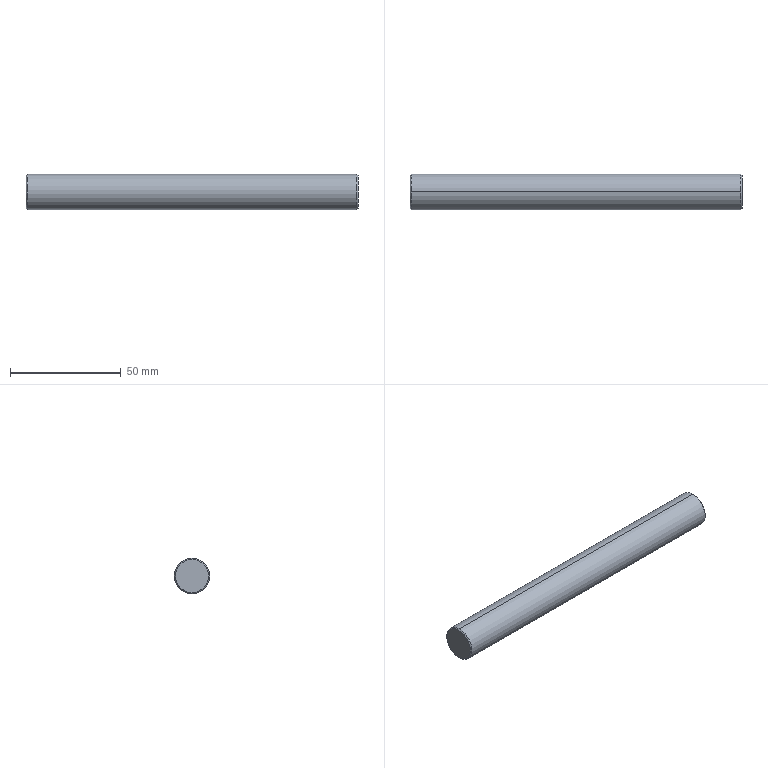Part | SolidWorks | features ICE 7, RevCut 2, Chamfer 1, Revolution 1 | 1 solid | 8 faces | box 150 x 16 x 16 mm | volume 30147 mm3 | cone 4 | cylinder 2 | plane 2 | commonest cylinder face diameters 16 x2
STEP:
#1=CARTESIAN_POINT('',(-75.,0.,7.5));
#2=VERTEX_POINT('',#1);
#3=CARTESIAN_POINT('',(-75.,0.,-7.5));
#4=VERTEX_POINT('',#3);
#5=CARTESIAN_POINT('',(-75.,0.,0.));
#6=DIRECTION('',(-1.,0.,0.));
#7=DIRECTION('',(0.,0.,-1.));
#8=AXIS2_PLACEMENT_3D('',#5,#6,#7);
#9=CIRCLE('',#8,7.5);
#10=EDGE_CURVE('',#2,#4,#9,.T.);
#11=ORIENTED_EDGE('',*,*,#10,.F.);
#12=CARTESIAN_POINT('',(-74.5,0.,8.));
#13=VERTEX_POINT('',#12);
#14=CARTESIAN_POINT('',(-75.,0.,7.5));
#15=DIRECTION('',(0.7071,0.,0.7071));
#16=VECTOR('',#15,1000.);
#17=LINE('',#14,#16);
#18=EDGE_CURVE('',#2,#13,#17,.T.);
#19=ORIENTED_EDGE('',*,*,#18,.T.);
#20=CARTESIAN_POINT('',(-74.5,0.,-8.));
#21=VERTEX_POINT('',#20);
#22=CARTESIAN_POINT('',(-74.5,0.,0.));
#23=DIRECTION('',(1.,0.,0.));
#24=DIRECTION('',(0.,0.,-1.));
#25=AXIS2_PLACEMENT_3D('',#22,#23,#24);
#26=CIRCLE('',#25,8.);
#27=EDGE_CURVE('',#21,#13,#26,.T.);
#28=ORIENTED_EDGE('',*,*,#27,.F.);
#29=CARTESIAN_POINT('',(-75.,0.,-7.5));
#30=DIRECTION('',(0.7071,0.,-0.7071));
#31=VECTOR('',#30,1000.);
#32=LINE('',#29,#31);
#33=EDGE_CURVE('',#4,#21,#32,.T.);
#34=ORIENTED_EDGE('',*,*,#33,.F.);
#35=EDGE_LOOP('',(#11,#19,#28,#34));
#36=FACE_OUTER_BOUND('',#35,.T.);
#37=CARTESIAN_POINT('',(-75.,0.,0.));
#38=DIRECTION('',(1.,0.,0.));
#39=DIRECTION('',(0.,0.,-1.));
#40=AXIS2_PLACEMENT_3D('',#37,#38,#39);
#41=CONICAL_SURFACE('',#40,7.5,0.7854);
#42=ADVANCED_FACE('',(#36),#41,.T.);
#43=CARTESIAN_POINT('',(75.,0.,-7.5));
#44=VERTEX_POINT('',#43);
#45=CARTESIAN_POINT('',(75.,0.,7.5));
#46=VERTEX_POINT('',#45);
#47=CARTESIAN_POINT('',(75.,0.,0.));
#48=DIRECTION('',(1.,0.,0.));
#49=DIRECTION('',(0.,0.,1.));
#50=AXIS2_PLACEMENT_3D('',#47,#48,#49);
#51=CIRCLE('',#50,7.5);
#52=EDGE_CURVE('',#44,#46,#51,.T.);
#53=ORIENTED_EDGE('',*,*,#52,.F.);
#54=CARTESIAN_POINT('',(74.5,0.,-8.));
#55=VERTEX_POINT('',#54);
#56=CARTESIAN_POINT('',(74.5,0.,-8.));
#57=DIRECTION('',(-0.7071,0.,-0.7071));
#58=VECTOR('',#57,1000.);
#59=LINE('',#56,#58);
#60=EDGE_CURVE('',#44,#55,#59,.T.);
#61=ORIENTED_EDGE('',*,*,#60,.T.);
#62=CARTESIAN_POINT('',(74.5,0.,8.));
#63=VERTEX_POINT('',#62);
#64=CARTESIAN_POINT('',(74.5,0.,0.));
#65=DIRECTION('',(-1.,0.,0.));
#66=DIRECTION('',(0.,0.,1.));
#67=AXIS2_PLACEMENT_3D('',#64,#65,#66);
#68=CIRCLE('',#67,8.);
#69=EDGE_CURVE('',#63,#55,#68,.T.);
#70=ORIENTED_EDGE('',*,*,#69,.F.);
#71=CARTESIAN_POINT('',(74.5,0.,8.));
#72=DIRECTION('',(-0.7071,0.,0.7071));
#73=VECTOR('',#72,1000.);
#74=LINE('',#71,#73);
#75=EDGE_CURVE('',#46,#63,#74,.T.);
#76=ORIENTED_EDGE('',*,*,#75,.F.);
#77=EDGE_LOOP('',(#53,#61,#70,#76));
#78=FACE_OUTER_BOUND('',#77,.T.);
#79=CARTESIAN_POINT('',(74.5,0.,0.));
#80=DIRECTION('',(-1.,0.,0.));
#81=DIRECTION('',(0.,0.,1.));
#82=AXIS2_PLACEMENT_3D('',#79,#80,#81);
#83=CONICAL_SURFACE('',#82,8.,0.7854);
#84=ADVANCED_FACE('',(#78),#83,.T.);
#85=ORIENTED_EDGE('',*,*,#69,.T.);
#86=CARTESIAN_POINT('',(0.,0.,-8.));
#87=DIRECTION('',(-1.,0.,0.));
#88=VECTOR('',#87,1000.);
#89=LINE('',#86,#88);
#90=EDGE_CURVE('',#55,#21,#89,.T.);
#91=ORIENTED_EDGE('',*,*,#90,.T.);
#92=ORIENTED_EDGE('',*,*,#27,.T.);
#93=CARTESIAN_POINT('',(0.,0.,8.));
#94=DIRECTION('',(-1.,0.,0.));
#95=VECTOR('',#94,1000.);
#96=LINE('',#93,#95);
#97=EDGE_CURVE('',#63,#13,#96,.T.);
#98=ORIENTED_EDGE('',*,*,#97,.F.);
#99=EDGE_LOOP('',(#85,#91,#92,#98));
#100=FACE_OUTER_BOUND('',#99,.T.);
#101=CARTESIAN_POINT('',(0.,0.,0.));
#102=DIRECTION('',(-1.,0.,0.));
#103=DIRECTION('',(0.,0.,1.));
#104=AXIS2_PLACEMENT_3D('',#101,#102,#103);
#105=CYLINDRICAL_SURFACE('',#104,8.);
#106=ADVANCED_FACE('',(#100),#105,.T.);
#107=CARTESIAN_POINT('',(-75.,0.,0.));
#108=DIRECTION('',(-1.,0.,0.));
#109=DIRECTION('',(0.,0.,-1.));
#110=AXIS2_PLACEMENT_3D('',#107,#108,#109);
#111=CIRCLE('',#110,7.5);
#112=EDGE_CURVE('',#4,#2,#111,.T.);
#113=ORIENTED_EDGE('',*,*,#112,.T.);
#114=ORIENTED_EDGE('',*,*,#10,.T.);
#115=EDGE_LOOP('',(#113,#114));
#116=FACE_OUTER_BOUND('',#115,.T.);
#117=CARTESIAN_POINT('',(-75.,8.,0.));
#118=DIRECTION('',(1.,0.,0.));
#119=DIRECTION('',(0.,0.,-1.));
#120=AXIS2_PLACEMENT_3D('',#117,#118,#119);
#121=PLANE('',#120);
#122=ADVANCED_FACE('',(#116),#121,.F.);
#123=CARTESIAN_POINT('',(75.,0.,0.));
#124=DIRECTION('',(1.,0.,0.));
#125=DIRECTION('',(0.,0.,1.));
#126=AXIS2_PLACEMENT_3D('',#123,#124,#125);
#127=CIRCLE('',#126,7.5);
#128=EDGE_CURVE('',#46,#44,#127,.T.);
#129=ORIENTED_EDGE('',*,*,#128,.T.);
#130=ORIENTED_EDGE('',*,*,#52,.T.);
#131=EDGE_LOOP('',(#129,#130));
#132=FACE_OUTER_BOUND('',#131,.T.);
#133=CARTESIAN_POINT('',(75.,8.,0.));
#134=DIRECTION('',(-1.,0.,0.));
#135=DIRECTION('',(0.,0.,1.));
#136=AXIS2_PLACEMENT_3D('',#133,#134,#135);
#137=PLANE('',#136);
#138=ADVANCED_FACE('',(#132),#137,.F.);
#139=ORIENTED_EDGE('',*,*,#90,.F.);
#140=CARTESIAN_POINT('',(74.5,0.,0.));
#141=DIRECTION('',(-1.,0.,0.));
#142=DIRECTION('',(0.,0.,1.));
#143=AXIS2_PLACEMENT_3D('',#140,#141,#142);
#144=CIRCLE('',#143,8.);
#145=EDGE_CURVE('',#55,#63,#144,.T.);
#146=ORIENTED_EDGE('',*,*,#145,.T.);
#147=ORIENTED_EDGE('',*,*,#97,.T.);
#148=CARTESIAN_POINT('',(-74.5,0.,0.));
#149=DIRECTION('',(1.,0.,0.));
#150=DIRECTION('',(0.,0.,-1.));
#151=AXIS2_PLACEMENT_3D('',#148,#149,#150);
#152=CIRCLE('',#151,8.);
#153=EDGE_CURVE('',#13,#21,#152,.T.);
#154=ORIENTED_EDGE('',*,*,#153,.T.);
#155=EDGE_LOOP('',(#139,#146,#147,#154));
#156=FACE_OUTER_BOUND('',#155,.T.);
#157=CARTESIAN_POINT('',(0.,0.,0.));
#158=DIRECTION('',(-1.,0.,0.));
#159=DIRECTION('',(0.,0.,1.));
#160=AXIS2_PLACEMENT_3D('',#157,#158,#159);
#161=CYLINDRICAL_SURFACE('',#160,8.);
#162=ADVANCED_FACE('',(#156),#161,.T.);
#163=ORIENTED_EDGE('',*,*,#60,.F.);
#164=ORIENTED_EDGE('',*,*,#128,.F.);
#165=ORIENTED_EDGE('',*,*,#75,.T.);
#166=ORIENTED_EDGE('',*,*,#145,.F.);
#167=EDGE_LOOP('',(#163,#164,#165,#166));
#168=FACE_OUTER_BOUND('',#167,.T.);
#169=CARTESIAN_POINT('',(74.5,0.,0.));
#170=DIRECTION('',(-1.,0.,0.));
#171=DIRECTION('',(0.,0.,1.));
#172=AXIS2_PLACEMENT_3D('',#169,#170,#171);
#173=CONICAL_SURFACE('',#172,8.,0.7854);
#174=ADVANCED_FACE('',(#168),#173,.T.);
#175=ORIENTED_EDGE('',*,*,#18,.F.);
#176=ORIENTED_EDGE('',*,*,#112,.F.);
#177=ORIENTED_EDGE('',*,*,#33,.T.);
#178=ORIENTED_EDGE('',*,*,#153,.F.);
#179=EDGE_LOOP('',(#175,#176,#177,#178));
#180=FACE_OUTER_BOUND('',#179,.T.);
#181=CARTESIAN_POINT('',(-75.,0.,0.));
#182=DIRECTION('',(1.,0.,0.));
#183=DIRECTION('',(0.,0.,-1.));
#184=AXIS2_PLACEMENT_3D('',#181,#182,#183);
#185=CONICAL_SURFACE('',#184,7.5,0.7854);
#186=ADVANCED_FACE('',(#180),#185,.T.);
#187=CLOSED_SHELL('',(#42,#84,#106,#122,#138,#162,#174,#186));
#188=MANIFOLD_SOLID_BREP('',#187);
#189=CARTESIAN_POINT('',(0.,0.,0.));
#190=DIRECTION('',(0.,0.,1.));
#191=DIRECTION('',(1.,0.,0.));
#192=AXIS2_PLACEMENT_3D('',#189,#190,#191);
#193=(LENGTH_UNIT()NAMED_UNIT(*)SI_UNIT(.MILLI.,.METRE.));
#194=UNCERTAINTY_MEASURE_WITH_UNIT(LENGTH_MEASURE(0.00001),#193,'','');
#195=(NAMED_UNIT(*)PLANE_ANGLE_UNIT()SI_UNIT($,.RADIAN.));
#196=(NAMED_UNIT(*)SI_UNIT($,.STERADIAN.)SOLID_ANGLE_UNIT());
#197=(GEOMETRIC_REPRESENTATION_CONTEXT(3)GLOBAL_UNCERTAINTY_ASSIGNED_CONTEXT((#194))GLOBAL_UNIT_ASSIGNED_CONTEXT((#193,#195,#196))REPRESENTATION_CONTEXT('',''));
#198=ADVANCED_BREP_SHAPE_REPRESENTATION('',(#188,#192),#197);